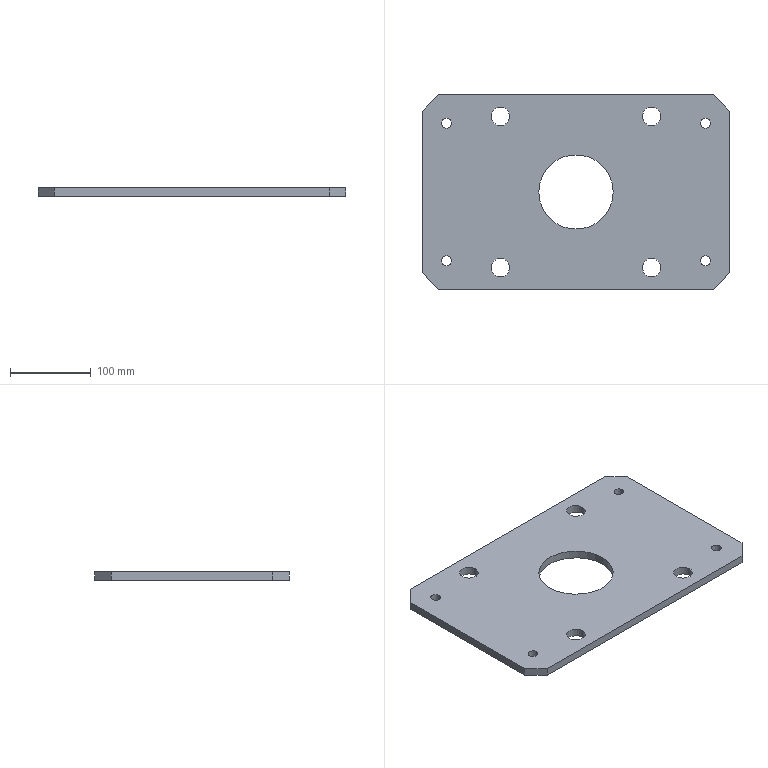Part | SolidWorks | features BaseBody 1 | 1 solid | 28 faces | box 380 x 240 x 10 mm | volume 816381 mm3 | cylinder 18 | plane 10 | commonest cylinder face diameters 12 x8 23 x8 92 x2
STEP:
#1=CARTESIAN_POINT('',(-154.,85.,10.));
#2=VERTEX_POINT('',#1);
#3=CARTESIAN_POINT('',(-166.,85.,10.));
#4=VERTEX_POINT('',#3);
#5=CARTESIAN_POINT('',(-160.,85.,10.));
#6=DIRECTION('',(0.,0.,-1.));
#7=DIRECTION('',(-1.,0.,0.));
#8=AXIS2_PLACEMENT_3D('',#5,#6,#7);
#9=CIRCLE('',#8,6.);
#10=EDGE_CURVE('',#2,#4,#9,.T.);
#11=ORIENTED_EDGE('',*,*,#10,.F.);
#12=CARTESIAN_POINT('',(-154.,85.,0.));
#13=VERTEX_POINT('',#12);
#14=CARTESIAN_POINT('',(-154.,85.,10.));
#15=DIRECTION('',(0.,0.,-1.));
#16=VECTOR('',#15,1000.);
#17=LINE('',#14,#16);
#18=EDGE_CURVE('',#2,#13,#17,.T.);
#19=ORIENTED_EDGE('',*,*,#18,.T.);
#20=CARTESIAN_POINT('',(-166.,85.,0.));
#21=VERTEX_POINT('',#20);
#22=CARTESIAN_POINT('',(-160.,85.,0.));
#23=DIRECTION('',(0.,0.,-1.));
#24=DIRECTION('',(-1.,0.,0.));
#25=AXIS2_PLACEMENT_3D('',#22,#23,#24);
#26=CIRCLE('',#25,6.);
#27=EDGE_CURVE('',#13,#21,#26,.T.);
#28=ORIENTED_EDGE('',*,*,#27,.T.);
#29=CARTESIAN_POINT('',(-166.,85.,10.));
#30=DIRECTION('',(0.,0.,-1.));
#31=VECTOR('',#30,1000.);
#32=LINE('',#29,#31);
#33=EDGE_CURVE('',#4,#21,#32,.T.);
#34=ORIENTED_EDGE('',*,*,#33,.F.);
#35=EDGE_LOOP('',(#11,#19,#28,#34));
#36=FACE_OUTER_BOUND('',#35,.T.);
#37=CARTESIAN_POINT('',(-160.,85.,10.));
#38=DIRECTION('',(0.,0.,-1.));
#39=DIRECTION('',(-1.,0.,0.));
#40=AXIS2_PLACEMENT_3D('',#37,#38,#39);
#41=CYLINDRICAL_SURFACE('',#40,6.);
#42=ADVANCED_FACE('',(#36),#41,.F.);
#43=CARTESIAN_POINT('',(-154.,-85.,10.));
#44=VERTEX_POINT('',#43);
#45=CARTESIAN_POINT('',(-166.,-85.,10.));
#46=VERTEX_POINT('',#45);
#47=CARTESIAN_POINT('',(-160.,-85.,10.));
#48=DIRECTION('',(0.,0.,-1.));
#49=DIRECTION('',(-1.,0.,0.));
#50=AXIS2_PLACEMENT_3D('',#47,#48,#49);
#51=CIRCLE('',#50,6.);
#52=EDGE_CURVE('',#44,#46,#51,.T.);
#53=ORIENTED_EDGE('',*,*,#52,.F.);
#54=CARTESIAN_POINT('',(-154.,-85.,0.));
#55=VERTEX_POINT('',#54);
#56=CARTESIAN_POINT('',(-154.,-85.,10.));
#57=DIRECTION('',(0.,0.,-1.));
#58=VECTOR('',#57,1000.);
#59=LINE('',#56,#58);
#60=EDGE_CURVE('',#44,#55,#59,.T.);
#61=ORIENTED_EDGE('',*,*,#60,.T.);
#62=CARTESIAN_POINT('',(-166.,-85.,0.));
#63=VERTEX_POINT('',#62);
#64=CARTESIAN_POINT('',(-160.,-85.,0.));
#65=DIRECTION('',(0.,0.,-1.));
#66=DIRECTION('',(-1.,0.,0.));
#67=AXIS2_PLACEMENT_3D('',#64,#65,#66);
#68=CIRCLE('',#67,6.);
#69=EDGE_CURVE('',#55,#63,#68,.T.);
#70=ORIENTED_EDGE('',*,*,#69,.T.);
#71=CARTESIAN_POINT('',(-166.,-85.,10.));
#72=DIRECTION('',(0.,0.,-1.));
#73=VECTOR('',#72,1000.);
#74=LINE('',#71,#73);
#75=EDGE_CURVE('',#46,#63,#74,.T.);
#76=ORIENTED_EDGE('',*,*,#75,.F.);
#77=EDGE_LOOP('',(#53,#61,#70,#76));
#78=FACE_OUTER_BOUND('',#77,.T.);
#79=CARTESIAN_POINT('',(-160.,-85.,10.));
#80=DIRECTION('',(0.,0.,-1.));
#81=DIRECTION('',(-1.,0.,0.));
#82=AXIS2_PLACEMENT_3D('',#79,#80,#81);
#83=CYLINDRICAL_SURFACE('',#82,6.);
#84=ADVANCED_FACE('',(#78),#83,.F.);
#85=CARTESIAN_POINT('',(166.,85.,10.));
#86=VERTEX_POINT('',#85);
#87=CARTESIAN_POINT('',(154.,85.,10.));
#88=VERTEX_POINT('',#87);
#89=CARTESIAN_POINT('',(160.,85.,10.));
#90=DIRECTION('',(0.,0.,-1.));
#91=DIRECTION('',(-1.,0.,0.));
#92=AXIS2_PLACEMENT_3D('',#89,#90,#91);
#93=CIRCLE('',#92,6.);
#94=EDGE_CURVE('',#86,#88,#93,.T.);
#95=ORIENTED_EDGE('',*,*,#94,.F.);
#96=CARTESIAN_POINT('',(166.,85.,0.));
#97=VERTEX_POINT('',#96);
#98=CARTESIAN_POINT('',(166.,85.,10.));
#99=DIRECTION('',(0.,0.,-1.));
#100=VECTOR('',#99,1000.);
#101=LINE('',#98,#100);
#102=EDGE_CURVE('',#86,#97,#101,.T.);
#103=ORIENTED_EDGE('',*,*,#102,.T.);
#104=CARTESIAN_POINT('',(154.,85.,0.));
#105=VERTEX_POINT('',#104);
#106=CARTESIAN_POINT('',(160.,85.,0.));
#107=DIRECTION('',(0.,0.,-1.));
#108=DIRECTION('',(-1.,0.,0.));
#109=AXIS2_PLACEMENT_3D('',#106,#107,#108);
#110=CIRCLE('',#109,6.);
#111=EDGE_CURVE('',#97,#105,#110,.T.);
#112=ORIENTED_EDGE('',*,*,#111,.T.);
#113=CARTESIAN_POINT('',(154.,85.,10.));
#114=DIRECTION('',(0.,0.,-1.));
#115=VECTOR('',#114,1000.);
#116=LINE('',#113,#115);
#117=EDGE_CURVE('',#88,#105,#116,.T.);
#118=ORIENTED_EDGE('',*,*,#117,.F.);
#119=EDGE_LOOP('',(#95,#103,#112,#118));
#120=FACE_OUTER_BOUND('',#119,.T.);
#121=CARTESIAN_POINT('',(160.,85.,10.));
#122=DIRECTION('',(0.,0.,-1.));
#123=DIRECTION('',(-1.,0.,0.));
#124=AXIS2_PLACEMENT_3D('',#121,#122,#123);
#125=CYLINDRICAL_SURFACE('',#124,6.);
#126=ADVANCED_FACE('',(#120),#125,.F.);
#127=CARTESIAN_POINT('',(166.,-85.,10.));
#128=VERTEX_POINT('',#127);
#129=CARTESIAN_POINT('',(154.,-85.,10.));
#130=VERTEX_POINT('',#129);
#131=CARTESIAN_POINT('',(160.,-85.,10.));
#132=DIRECTION('',(0.,0.,-1.));
#133=DIRECTION('',(-1.,0.,0.));
#134=AXIS2_PLACEMENT_3D('',#131,#132,#133);
#135=CIRCLE('',#134,6.);
#136=EDGE_CURVE('',#128,#130,#135,.T.);
#137=ORIENTED_EDGE('',*,*,#136,.F.);
#138=CARTESIAN_POINT('',(166.,-85.,0.));
#139=VERTEX_POINT('',#138);
#140=CARTESIAN_POINT('',(166.,-85.,10.));
#141=DIRECTION('',(0.,0.,-1.));
#142=VECTOR('',#141,1000.);
#143=LINE('',#140,#142);
#144=EDGE_CURVE('',#128,#139,#143,.T.);
#145=ORIENTED_EDGE('',*,*,#144,.T.);
#146=CARTESIAN_POINT('',(154.,-85.,0.));
#147=VERTEX_POINT('',#146);
#148=CARTESIAN_POINT('',(160.,-85.,0.));
#149=DIRECTION('',(0.,0.,-1.));
#150=DIRECTION('',(-1.,0.,0.));
#151=AXIS2_PLACEMENT_3D('',#148,#149,#150);
#152=CIRCLE('',#151,6.);
#153=EDGE_CURVE('',#139,#147,#152,.T.);
#154=ORIENTED_EDGE('',*,*,#153,.T.);
#155=CARTESIAN_POINT('',(154.,-85.,10.));
#156=DIRECTION('',(0.,0.,-1.));
#157=VECTOR('',#156,1000.);
#158=LINE('',#155,#157);
#159=EDGE_CURVE('',#130,#147,#158,.T.);
#160=ORIENTED_EDGE('',*,*,#159,.F.);
#161=EDGE_LOOP('',(#137,#145,#154,#160));
#162=FACE_OUTER_BOUND('',#161,.T.);
#163=CARTESIAN_POINT('',(160.,-85.,10.));
#164=DIRECTION('',(0.,0.,-1.));
#165=DIRECTION('',(-1.,0.,0.));
#166=AXIS2_PLACEMENT_3D('',#163,#164,#165);
#167=CYLINDRICAL_SURFACE('',#166,6.);
#168=ADVANCED_FACE('',(#162),#167,.F.);
#169=CARTESIAN_POINT('',(-82.,93.5,10.));
#170=VERTEX_POINT('',#169);
#171=CARTESIAN_POINT('',(-105.,93.5,10.));
#172=VERTEX_POINT('',#171);
#173=CARTESIAN_POINT('',(-93.5,93.5,10.));
#174=DIRECTION('',(0.,0.,-1.));
#175=DIRECTION('',(-1.,0.,0.));
#176=AXIS2_PLACEMENT_3D('',#173,#174,#175);
#177=CIRCLE('',#176,11.5);
#178=EDGE_CURVE('',#170,#172,#177,.T.);
#179=ORIENTED_EDGE('',*,*,#178,.F.);
#180=CARTESIAN_POINT('',(-82.,93.5,0.));
#181=VERTEX_POINT('',#180);
#182=CARTESIAN_POINT('',(-82.,93.5,10.));
#183=DIRECTION('',(0.,0.,-1.));
#184=VECTOR('',#183,1000.);
#185=LINE('',#182,#184);
#186=EDGE_CURVE('',#170,#181,#185,.T.);
#187=ORIENTED_EDGE('',*,*,#186,.T.);
#188=CARTESIAN_POINT('',(-105.,93.5,0.));
#189=VERTEX_POINT('',#188);
#190=CARTESIAN_POINT('',(-93.5,93.5,0.));
#191=DIRECTION('',(0.,0.,-1.));
#192=DIRECTION('',(-1.,0.,0.));
#193=AXIS2_PLACEMENT_3D('',#190,#191,#192);
#194=CIRCLE('',#193,11.5);
#195=EDGE_CURVE('',#181,#189,#194,.T.);
#196=ORIENTED_EDGE('',*,*,#195,.T.);
#197=CARTESIAN_POINT('',(-105.,93.5,10.));
#198=DIRECTION('',(0.,0.,-1.));
#199=VECTOR('',#198,1000.);
#200=LINE('',#197,#199);
#201=EDGE_CURVE('',#172,#189,#200,.T.);
#202=ORIENTED_EDGE('',*,*,#201,.F.);
#203=EDGE_LOOP('',(#179,#187,#196,#202));
#204=FACE_OUTER_BOUND('',#203,.T.);
#205=CARTESIAN_POINT('',(-93.5,93.5,10.));
#206=DIRECTION('',(0.,0.,-1.));
#207=DIRECTION('',(-1.,0.,0.));
#208=AXIS2_PLACEMENT_3D('',#205,#206,#207);
#209=CYLINDRICAL_SURFACE('',#208,11.5);
#210=ADVANCED_FACE('',(#204),#209,.F.);
#211=CARTESIAN_POINT('',(-82.,-93.5,10.));
#212=VERTEX_POINT('',#211);
#213=CARTESIAN_POINT('',(-105.,-93.5,10.));
#214=VERTEX_POINT('',#213);
#215=CARTESIAN_POINT('',(-93.5,-93.5,10.));
#216=DIRECTION('',(0.,0.,-1.));
#217=DIRECTION('',(-1.,0.,0.));
#218=AXIS2_PLACEMENT_3D('',#215,#216,#217);
#219=CIRCLE('',#218,11.5);
#220=EDGE_CURVE('',#212,#214,#219,.T.);
#221=ORIENTED_EDGE('',*,*,#220,.F.);
#222=CARTESIAN_POINT('',(-82.,-93.5,0.));
#223=VERTEX_POINT('',#222);
#224=CARTESIAN_POINT('',(-82.,-93.5,10.));
#225=DIRECTION('',(0.,0.,-1.));
#226=VECTOR('',#225,1000.);
#227=LINE('',#224,#226);
#228=EDGE_CURVE('',#212,#223,#227,.T.);
#229=ORIENTED_EDGE('',*,*,#228,.T.);
#230=CARTESIAN_POINT('',(-105.,-93.5,0.));
#231=VERTEX_POINT('',#230);
#232=CARTESIAN_POINT('',(-93.5,-93.5,0.));
#233=DIRECTION('',(0.,0.,-1.));
#234=DIRECTION('',(-1.,0.,0.));
#235=AXIS2_PLACEMENT_3D('',#232,#233,#234);
#236=CIRCLE('',#235,11.5);
#237=EDGE_CURVE('',#223,#231,#236,.T.);
#238=ORIENTED_EDGE('',*,*,#237,.T.);
#239=CARTESIAN_POINT('',(-105.,-93.5,10.));
#240=DIRECTION('',(0.,0.,-1.));
#241=VECTOR('',#240,1000.);
#242=LINE('',#239,#241);
#243=EDGE_CURVE('',#214,#231,#242,.T.);
#244=ORIENTED_EDGE('',*,*,#243,.F.);
#245=EDGE_LOOP('',(#221,#229,#238,#244));
#246=FACE_OUTER_BOUND('',#245,.T.);
#247=CARTESIAN_POINT('',(-93.5,-93.5,10.));
#248=DIRECTION('',(0.,0.,-1.));
#249=DIRECTION('',(-1.,0.,0.));
#250=AXIS2_PLACEMENT_3D('',#247,#248,#249);
#251=CYLINDRICAL_SURFACE('',#250,11.5);
#252=ADVANCED_FACE('',(#246),#251,.F.);
#253=CARTESIAN_POINT('',(105.,93.5,10.));
#254=VERTEX_POINT('',#253);
#255=CARTESIAN_POINT('',(82.,93.5,10.));
#256=VERTEX_POINT('',#255);
#257=CARTESIAN_POINT('',(93.5,93.5,10.));
#258=DIRECTION('',(0.,0.,-1.));
#259=DIRECTION('',(-1.,0.,0.));
#260=AXIS2_PLACEMENT_3D('',#257,#258,#259);
#261=CIRCLE('',#260,11.5);
#262=EDGE_CURVE('',#254,#256,#261,.T.);
#263=ORIENTED_EDGE('',*,*,#262,.F.);
#264=CARTESIAN_POINT('',(105.,93.5,0.));
#265=VERTEX_POINT('',#264);
#266=CARTESIAN_POINT('',(105.,93.5,10.));
#267=DIRECTION('',(0.,0.,-1.));
#268=VECTOR('',#267,1000.);
#269=LINE('',#266,#268);
#270=EDGE_CURVE('',#254,#265,#269,.T.);
#271=ORIENTED_EDGE('',*,*,#270,.T.);
#272=CARTESIAN_POINT('',(82.,93.5,0.));
#273=VERTEX_POINT('',#272);
#274=CARTESIAN_POINT('',(93.5,93.5,0.));
#275=DIRECTION('',(0.,0.,-1.));
#276=DIRECTION('',(-1.,0.,0.));
#277=AXIS2_PLACEMENT_3D('',#274,#275,#276);
#278=CIRCLE('',#277,11.5);
#279=EDGE_CURVE('',#265,#273,#278,.T.);
#280=ORIENTED_EDGE('',*,*,#279,.T.);
#281=CARTESIAN_POINT('',(82.,93.5,10.));
#282=DIRECTION('',(0.,0.,-1.));
#283=VECTOR('',#282,1000.);
#284=LINE('',#281,#283);
#285=EDGE_CURVE('',#256,#273,#284,.T.);
#286=ORIENTED_EDGE('',*,*,#285,.F.);
#287=EDGE_LOOP('',(#263,#271,#280,#286));
#288=FACE_OUTER_BOUND('',#287,.T.);
#289=CARTESIAN_POINT('',(93.5,93.5,10.));
#290=DIRECTION('',(0.,0.,-1.));
#291=DIRECTION('',(-1.,0.,0.));
#292=AXIS2_PLACEMENT_3D('',#289,#290,#291);
#293=CYLINDRICAL_SURFACE('',#292,11.5);
#294=ADVANCED_FACE('',(#288),#293,.F.);
#295=CARTESIAN_POINT('',(105.,-93.5,10.));
#296=VERTEX_POINT('',#295);
#297=CARTESIAN_POINT('',(82.,-93.5,10.));
#298=VERTEX_POINT('',#297);
#299=CARTESIAN_POINT('',(93.5,-93.5,10.));
#300=DIRECTION('',(0.,0.,-1.));
#301=DIRECTION('',(-1.,0.,0.));
#302=AXIS2_PLACEMENT_3D('',#299,#300,#301);
#303=CIRCLE('',#302,11.5);
#304=EDGE_CURVE('',#296,#298,#303,.T.);
#305=ORIENTED_EDGE('',*,*,#304,.F.);
#306=CARTESIAN_POINT('',(105.,-93.5,0.));
#307=VERTEX_POINT('',#306);
#308=CARTESIAN_POINT('',(105.,-93.5,10.));
#309=DIRECTION('',(0.,0.,-1.));
#310=VECTOR('',#309,1000.);
#311=LINE('',#308,#310);
#312=EDGE_CURVE('',#296,#307,#311,.T.);
#313=ORIENTED_EDGE('',*,*,#312,.T.);
#314=CARTESIAN_POINT('',(82.,-93.5,0.));
#315=VERTEX_POINT('',#314);
#316=CARTESIAN_POINT('',(93.5,-93.5,0.));
#317=DIRECTION('',(0.,0.,-1.));
#318=DIRECTION('',(-1.,0.,0.));
#319=AXIS2_PLACEMENT_3D('',#316,#317,#318);
#320=CIRCLE('',#319,11.5);
#321=EDGE_CURVE('',#307,#315,#320,.T.);
#322=ORIENTED_EDGE('',*,*,#321,.T.);
#323=CARTESIAN_POINT('',(82.,-93.5,10.));
#324=DIRECTION('',(0.,0.,-1.));
#325=VECTOR('',#324,1000.);
#326=LINE('',#323,#325);
#327=EDGE_CURVE('',#298,#315,#326,.T.);
#328=ORIENTED_EDGE('',*,*,#327,.F.);
#329=EDGE_LOOP('',(#305,#313,#322,#328));
#330=FACE_OUTER_BOUND('',#329,.T.);
#331=CARTESIAN_POINT('',(93.5,-93.5,10.));
#332=DIRECTION('',(0.,0.,-1.));
#333=DIRECTION('',(-1.,0.,0.));
#334=AXIS2_PLACEMENT_3D('',#331,#332,#333);
#335=CYLINDRICAL_SURFACE('',#334,11.5);
#336=ADVANCED_FACE('',(#330),#335,.F.);
#337=CARTESIAN_POINT('',(46.,0.,10.));
#338=VERTEX_POINT('',#337);
#339=CARTESIAN_POINT('',(-46.,0.,10.));
#340=VERTEX_POINT('',#339);
#341=CARTESIAN_POINT('',(0.,0.,10.));
#342=DIRECTION('',(0.,0.,-1.));
#343=DIRECTION('',(-1.,0.,0.));
#344=AXIS2_PLACEMENT_3D('',#341,#342,#343);
#345=CIRCLE('',#344,46.);
#346=EDGE_CURVE('',#338,#340,#345,.T.);
#347=ORIENTED_EDGE('',*,*,#346,.F.);
#348=CARTESIAN_POINT('',(46.,0.,0.));
#349=VERTEX_POINT('',#348);
#350=CARTESIAN_POINT('',(46.,0.,10.));
#351=DIRECTION('',(0.,0.,-1.));
#352=VECTOR('',#351,1000.);
#353=LINE('',#350,#352);
#354=EDGE_CURVE('',#338,#349,#353,.T.);
#355=ORIENTED_EDGE('',*,*,#354,.T.);
#356=CARTESIAN_POINT('',(-46.,0.,0.));
#357=VERTEX_POINT('',#356);
#358=CARTESIAN_POINT('',(0.,0.,0.));
#359=DIRECTION('',(0.,0.,-1.));
#360=DIRECTION('',(-1.,0.,0.));
#361=AXIS2_PLACEMENT_3D('',#358,#359,#360);
#362=CIRCLE('',#361,46.);
#363=EDGE_CURVE('',#349,#357,#362,.T.);
#364=ORIENTED_EDGE('',*,*,#363,.T.);
#365=CARTESIAN_POINT('',(-46.,0.,10.));
#366=DIRECTION('',(0.,0.,-1.));
#367=VECTOR('',#366,1000.);
#368=LINE('',#365,#367);
#369=EDGE_CURVE('',#340,#357,#368,.T.);
#370=ORIENTED_EDGE('',*,*,#369,.F.);
#371=EDGE_LOOP('',(#347,#355,#364,#370));
#372=FACE_OUTER_BOUND('',#371,.T.);
#373=CARTESIAN_POINT('',(0.,0.,10.));
#374=DIRECTION('',(0.,0.,-1.));
#375=DIRECTION('',(-1.,0.,0.));
#376=AXIS2_PLACEMENT_3D('',#373,#374,#375);
#377=CYLINDRICAL_SURFACE('',#376,46.);
#378=ADVANCED_FACE('',(#372),#377,.F.);
#379=CARTESIAN_POINT('',(-160.,85.,0.));
#380=DIRECTION('',(0.,0.,-1.));
#381=DIRECTION('',(-1.,0.,0.));
#382=AXIS2_PLACEMENT_3D('',#379,#380,#381);
#383=CIRCLE('',#382,6.);
#384=EDGE_CURVE('',#21,#13,#383,.T.);
#385=ORIENTED_EDGE('',*,*,#384,.F.);
#386=ORIENTED_EDGE('',*,*,#27,.F.);
#387=EDGE_LOOP('',(#385,#386));
#388=FACE_BOUND('',#387,.T.);
#389=CARTESIAN_POINT('',(-160.,-85.,0.));
#390=DIRECTION('',(0.,0.,-1.));
#391=DIRECTION('',(-1.,0.,0.));
#392=AXIS2_PLACEMENT_3D('',#389,#390,#391);
#393=CIRCLE('',#392,6.);
#394=EDGE_CURVE('',#63,#55,#393,.T.);
#395=ORIENTED_EDGE('',*,*,#394,.F.);
#396=ORIENTED_EDGE('',*,*,#69,.F.);
#397=EDGE_LOOP('',(#395,#396));
#398=FACE_BOUND('',#397,.T.);
#399=CARTESIAN_POINT('',(160.,85.,0.));
#400=DIRECTION('',(0.,0.,-1.));
#401=DIRECTION('',(-1.,0.,0.));
#402=AXIS2_PLACEMENT_3D('',#399,#400,#401);
#403=CIRCLE('',#402,6.);
#404=EDGE_CURVE('',#105,#97,#403,.T.);
#405=ORIENTED_EDGE('',*,*,#404,.F.);
#406=ORIENTED_EDGE('',*,*,#111,.F.);
#407=EDGE_LOOP('',(#405,#406));
#408=FACE_BOUND('',#407,.T.);
#409=CARTESIAN_POINT('',(160.,-85.,0.));
#410=DIRECTION('',(0.,0.,-1.));
#411=DIRECTION('',(-1.,0.,0.));
#412=AXIS2_PLACEMENT_3D('',#409,#410,#411);
#413=CIRCLE('',#412,6.);
#414=EDGE_CURVE('',#147,#139,#413,.T.);
#415=ORIENTED_EDGE('',*,*,#414,.F.);
#416=ORIENTED_EDGE('',*,*,#153,.F.);
#417=EDGE_LOOP('',(#415,#416));
#418=FACE_BOUND('',#417,.T.);
#419=CARTESIAN_POINT('',(-93.5,93.5,0.));
#420=DIRECTION('',(0.,0.,-1.));
#421=DIRECTION('',(-1.,0.,0.));
#422=AXIS2_PLACEMENT_3D('',#419,#420,#421);
#423=CIRCLE('',#422,11.5);
#424=EDGE_CURVE('',#189,#181,#423,.T.);
#425=ORIENTED_EDGE('',*,*,#424,.F.);
#426=ORIENTED_EDGE('',*,*,#195,.F.);
#427=EDGE_LOOP('',(#425,#426));
#428=FACE_BOUND('',#427,.T.);
#429=CARTESIAN_POINT('',(-93.5,-93.5,0.));
#430=DIRECTION('',(0.,0.,-1.));
#431=DIRECTION('',(-1.,0.,0.));
#432=AXIS2_PLACEMENT_3D('',#429,#430,#431);
#433=CIRCLE('',#432,11.5);
#434=EDGE_CURVE('',#231,#223,#433,.T.);
#435=ORIENTED_EDGE('',*,*,#434,.F.);
#436=ORIENTED_EDGE('',*,*,#237,.F.);
#437=EDGE_LOOP('',(#435,#436));
#438=FACE_BOUND('',#437,.T.);
#439=CARTESIAN_POINT('',(93.5,93.5,0.));
#440=DIRECTION('',(0.,0.,-1.));
#441=DIRECTION('',(-1.,0.,0.));
#442=AXIS2_PLACEMENT_3D('',#439,#440,#441);
#443=CIRCLE('',#442,11.5);
#444=EDGE_CURVE('',#273,#265,#443,.T.);
#445=ORIENTED_EDGE('',*,*,#444,.F.);
#446=ORIENTED_EDGE('',*,*,#279,.F.);
#447=EDGE_LOOP('',(#445,#446));
#448=FACE_BOUND('',#447,.T.);
#449=CARTESIAN_POINT('',(93.5,-93.5,0.));
#450=DIRECTION('',(0.,0.,-1.));
#451=DIRECTION('',(-1.,0.,0.));
#452=AXIS2_PLACEMENT_3D('',#449,#450,#451);
#453=CIRCLE('',#452,11.5);
#454=EDGE_CURVE('',#315,#307,#453,.T.);
#455=ORIENTED_EDGE('',*,*,#454,.F.);
#456=ORIENTED_EDGE('',*,*,#321,.F.);
#457=EDGE_LOOP('',(#455,#456));
#458=FACE_BOUND('',#457,.T.);
#459=CARTESIAN_POINT('',(0.,0.,0.));
#460=DIRECTION('',(0.,0.,-1.));
#461=DIRECTION('',(-1.,0.,0.));
#462=AXIS2_PLACEMENT_3D('',#459,#460,#461);
#463=CIRCLE('',#462,46.);
#464=EDGE_CURVE('',#357,#349,#463,.T.);
#465=ORIENTED_EDGE('',*,*,#464,.F.);
#466=ORIENTED_EDGE('',*,*,#363,.F.);
#467=EDGE_LOOP('',(#465,#466));
#468=FACE_BOUND('',#467,.T.);
#469=CARTESIAN_POINT('',(170.,-120.,0.));
#470=VERTEX_POINT('',#469);
#471=CARTESIAN_POINT('',(190.,-100.,0.));
#472=VERTEX_POINT('',#471);
#473=CARTESIAN_POINT('',(170.,-120.,0.));
#474=DIRECTION('',(0.7071,0.7071,0.));
#475=VECTOR('',#474,1000.);
#476=LINE('',#473,#475);
#477=EDGE_CURVE('',#470,#472,#476,.T.);
#478=ORIENTED_EDGE('',*,*,#477,.F.);
#479=CARTESIAN_POINT('',(-170.,-120.,0.));
#480=VERTEX_POINT('',#479);
#481=CARTESIAN_POINT('',(0.,-120.,0.));
#482=DIRECTION('',(1.,0.,0.));
#483=VECTOR('',#482,1000.);
#484=LINE('',#481,#483);
#485=EDGE_CURVE('',#480,#470,#484,.T.);
#486=ORIENTED_EDGE('',*,*,#485,.F.);
#487=CARTESIAN_POINT('',(-190.,-100.,0.));
#488=VERTEX_POINT('',#487);
#489=CARTESIAN_POINT('',(-190.,-100.,0.));
#490=DIRECTION('',(0.7071,-0.7071,0.));
#491=VECTOR('',#490,1000.);
#492=LINE('',#489,#491);
#493=EDGE_CURVE('',#488,#480,#492,.T.);
#494=ORIENTED_EDGE('',*,*,#493,.F.);
#495=CARTESIAN_POINT('',(-190.,100.,0.));
#496=VERTEX_POINT('',#495);
#497=CARTESIAN_POINT('',(-190.,0.,0.));
#498=DIRECTION('',(0.,-1.,0.));
#499=VECTOR('',#498,1000.);
#500=LINE('',#497,#499);
#501=EDGE_CURVE('',#496,#488,#500,.T.);
#502=ORIENTED_EDGE('',*,*,#501,.F.);
#503=CARTESIAN_POINT('',(-170.,120.,0.));
#504=VERTEX_POINT('',#503);
#505=CARTESIAN_POINT('',(-170.,120.,0.));
#506=DIRECTION('',(-0.7071,-0.7071,0.));
#507=VECTOR('',#506,1000.);
#508=LINE('',#505,#507);
#509=EDGE_CURVE('',#504,#496,#508,.T.);
#510=ORIENTED_EDGE('',*,*,#509,.F.);
#511=CARTESIAN_POINT('',(170.,120.,0.));
#512=VERTEX_POINT('',#511);
#513=CARTESIAN_POINT('',(0.,120.,0.));
#514=DIRECTION('',(-1.,0.,0.));
#515=VECTOR('',#514,1000.);
#516=LINE('',#513,#515);
#517=EDGE_CURVE('',#512,#504,#516,.T.);
#518=ORIENTED_EDGE('',*,*,#517,.F.);
#519=CARTESIAN_POINT('',(190.,100.,0.));
#520=VERTEX_POINT('',#519);
#521=CARTESIAN_POINT('',(190.,100.,0.));
#522=DIRECTION('',(-0.7071,0.7071,0.));
#523=VECTOR('',#522,1000.);
#524=LINE('',#521,#523);
#525=EDGE_CURVE('',#520,#512,#524,.T.);
#526=ORIENTED_EDGE('',*,*,#525,.F.);
#527=CARTESIAN_POINT('',(190.,0.,0.));
#528=DIRECTION('',(0.,1.,0.));
#529=VECTOR('',#528,1000.);
#530=LINE('',#527,#529);
#531=EDGE_CURVE('',#472,#520,#530,.T.);
#532=ORIENTED_EDGE('',*,*,#531,.F.);
#533=EDGE_LOOP('',(#478,#486,#494,#502,#510,#518,#526,#532));
#534=FACE_OUTER_BOUND('',#533,.T.);
#535=CARTESIAN_POINT('',(0.,0.,0.));
#536=DIRECTION('',(0.,0.,1.));
#537=DIRECTION('',(1.,0.,0.));
#538=AXIS2_PLACEMENT_3D('',#535,#536,#537);
#539=PLANE('',#538);
#540=ADVANCED_FACE('',(#388,#398,#408,#418,#428,#438,#448,#458,#468,#534),#539,.F.);
#541=ORIENTED_EDGE('',*,*,#18,.F.);
#542=CARTESIAN_POINT('',(-160.,85.,10.));
#543=DIRECTION('',(0.,0.,-1.));
#544=DIRECTION('',(-1.,0.,0.));
#545=AXIS2_PLACEMENT_3D('',#542,#543,#544);
#546=CIRCLE('',#545,6.);
#547=EDGE_CURVE('',#4,#2,#546,.T.);
#548=ORIENTED_EDGE('',*,*,#547,.F.);
#549=ORIENTED_EDGE('',*,*,#33,.T.);
#550=ORIENTED_EDGE('',*,*,#384,.T.);
#551=EDGE_LOOP('',(#541,#548,#549,#550));
#552=FACE_OUTER_BOUND('',#551,.T.);
#553=CARTESIAN_POINT('',(-160.,85.,10.));
#554=DIRECTION('',(0.,0.,-1.));
#555=DIRECTION('',(-1.,0.,0.));
#556=AXIS2_PLACEMENT_3D('',#553,#554,#555);
#557=CYLINDRICAL_SURFACE('',#556,6.);
#558=ADVANCED_FACE('',(#552),#557,.F.);
#559=ORIENTED_EDGE('',*,*,#60,.F.);
#560=CARTESIAN_POINT('',(-160.,-85.,10.));
#561=DIRECTION('',(0.,0.,-1.));
#562=DIRECTION('',(-1.,0.,0.));
#563=AXIS2_PLACEMENT_3D('',#560,#561,#562);
#564=CIRCLE('',#563,6.);
#565=EDGE_CURVE('',#46,#44,#564,.T.);
#566=ORIENTED_EDGE('',*,*,#565,.F.);
#567=ORIENTED_EDGE('',*,*,#75,.T.);
#568=ORIENTED_EDGE('',*,*,#394,.T.);
#569=EDGE_LOOP('',(#559,#566,#567,#568));
#570=FACE_OUTER_BOUND('',#569,.T.);
#571=CARTESIAN_POINT('',(-160.,-85.,10.));
#572=DIRECTION('',(0.,0.,-1.));
#573=DIRECTION('',(-1.,0.,0.));
#574=AXIS2_PLACEMENT_3D('',#571,#572,#573);
#575=CYLINDRICAL_SURFACE('',#574,6.);
#576=ADVANCED_FACE('',(#570),#575,.F.);
#577=ORIENTED_EDGE('',*,*,#102,.F.);
#578=CARTESIAN_POINT('',(160.,85.,10.));
#579=DIRECTION('',(0.,0.,-1.));
#580=DIRECTION('',(-1.,0.,0.));
#581=AXIS2_PLACEMENT_3D('',#578,#579,#580);
#582=CIRCLE('',#581,6.);
#583=EDGE_CURVE('',#88,#86,#582,.T.);
#584=ORIENTED_EDGE('',*,*,#583,.F.);
#585=ORIENTED_EDGE('',*,*,#117,.T.);
#586=ORIENTED_EDGE('',*,*,#404,.T.);
#587=EDGE_LOOP('',(#577,#584,#585,#586));
#588=FACE_OUTER_BOUND('',#587,.T.);
#589=CARTESIAN_POINT('',(160.,85.,10.));
#590=DIRECTION('',(0.,0.,-1.));
#591=DIRECTION('',(-1.,0.,0.));
#592=AXIS2_PLACEMENT_3D('',#589,#590,#591);
#593=CYLINDRICAL_SURFACE('',#592,6.);
#594=ADVANCED_FACE('',(#588),#593,.F.);
#595=ORIENTED_EDGE('',*,*,#144,.F.);
#596=CARTESIAN_POINT('',(160.,-85.,10.));
#597=DIRECTION('',(0.,0.,-1.));
#598=DIRECTION('',(-1.,0.,0.));
#599=AXIS2_PLACEMENT_3D('',#596,#597,#598);
#600=CIRCLE('',#599,6.);
#601=EDGE_CURVE('',#130,#128,#600,.T.);
#602=ORIENTED_EDGE('',*,*,#601,.F.);
#603=ORIENTED_EDGE('',*,*,#159,.T.);
#604=ORIENTED_EDGE('',*,*,#414,.T.);
#605=EDGE_LOOP('',(#595,#602,#603,#604));
#606=FACE_OUTER_BOUND('',#605,.T.);
#607=CARTESIAN_POINT('',(160.,-85.,10.));
#608=DIRECTION('',(0.,0.,-1.));
#609=DIRECTION('',(-1.,0.,0.));
#610=AXIS2_PLACEMENT_3D('',#607,#608,#609);
#611=CYLINDRICAL_SURFACE('',#610,6.);
#612=ADVANCED_FACE('',(#606),#611,.F.);
#613=ORIENTED_EDGE('',*,*,#186,.F.);
#614=CARTESIAN_POINT('',(-93.5,93.5,10.));
#615=DIRECTION('',(0.,0.,-1.));
#616=DIRECTION('',(-1.,0.,0.));
#617=AXIS2_PLACEMENT_3D('',#614,#615,#616);
#618=CIRCLE('',#617,11.5);
#619=EDGE_CURVE('',#172,#170,#618,.T.);
#620=ORIENTED_EDGE('',*,*,#619,.F.);
#621=ORIENTED_EDGE('',*,*,#201,.T.);
#622=ORIENTED_EDGE('',*,*,#424,.T.);
#623=EDGE_LOOP('',(#613,#620,#621,#622));
#624=FACE_OUTER_BOUND('',#623,.T.);
#625=CARTESIAN_POINT('',(-93.5,93.5,10.));
#626=DIRECTION('',(0.,0.,-1.));
#627=DIRECTION('',(-1.,0.,0.));
#628=AXIS2_PLACEMENT_3D('',#625,#626,#627);
#629=CYLINDRICAL_SURFACE('',#628,11.5);
#630=ADVANCED_FACE('',(#624),#629,.F.);
#631=ORIENTED_EDGE('',*,*,#228,.F.);
#632=CARTESIAN_POINT('',(-93.5,-93.5,10.));
#633=DIRECTION('',(0.,0.,-1.));
#634=DIRECTION('',(-1.,0.,0.));
#635=AXIS2_PLACEMENT_3D('',#632,#633,#634);
#636=CIRCLE('',#635,11.5);
#637=EDGE_CURVE('',#214,#212,#636,.T.);
#638=ORIENTED_EDGE('',*,*,#637,.F.);
#639=ORIENTED_EDGE('',*,*,#243,.T.);
#640=ORIENTED_EDGE('',*,*,#434,.T.);
#641=EDGE_LOOP('',(#631,#638,#639,#640));
#642=FACE_OUTER_BOUND('',#641,.T.);
#643=CARTESIAN_POINT('',(-93.5,-93.5,10.));
#644=DIRECTION('',(0.,0.,-1.));
#645=DIRECTION('',(-1.,0.,0.));
#646=AXIS2_PLACEMENT_3D('',#643,#644,#645);
#647=CYLINDRICAL_SURFACE('',#646,11.5);
#648=ADVANCED_FACE('',(#642),#647,.F.);
#649=ORIENTED_EDGE('',*,*,#270,.F.);
#650=CARTESIAN_POINT('',(93.5,93.5,10.));
#651=DIRECTION('',(0.,0.,-1.));
#652=DIRECTION('',(-1.,0.,0.));
#653=AXIS2_PLACEMENT_3D('',#650,#651,#652);
#654=CIRCLE('',#653,11.5);
#655=EDGE_CURVE('',#256,#254,#654,.T.);
#656=ORIENTED_EDGE('',*,*,#655,.F.);
#657=ORIENTED_EDGE('',*,*,#285,.T.);
#658=ORIENTED_EDGE('',*,*,#444,.T.);
#659=EDGE_LOOP('',(#649,#656,#657,#658));
#660=FACE_OUTER_BOUND('',#659,.T.);
#661=CARTESIAN_POINT('',(93.5,93.5,10.));
#662=DIRECTION('',(0.,0.,-1.));
#663=DIRECTION('',(-1.,0.,0.));
#664=AXIS2_PLACEMENT_3D('',#661,#662,#663);
#665=CYLINDRICAL_SURFACE('',#664,11.5);
#666=ADVANCED_FACE('',(#660),#665,.F.);
#667=ORIENTED_EDGE('',*,*,#312,.F.);
#668=CARTESIAN_POINT('',(93.5,-93.5,10.));
#669=DIRECTION('',(0.,0.,-1.));
#670=DIRECTION('',(-1.,0.,0.));
#671=AXIS2_PLACEMENT_3D('',#668,#669,#670);
#672=CIRCLE('',#671,11.5);
#673=EDGE_CURVE('',#298,#296,#672,.T.);
#674=ORIENTED_EDGE('',*,*,#673,.F.);
#675=ORIENTED_EDGE('',*,*,#327,.T.);
#676=ORIENTED_EDGE('',*,*,#454,.T.);
#677=EDGE_LOOP('',(#667,#674,#675,#676));
#678=FACE_OUTER_BOUND('',#677,.T.);
#679=CARTESIAN_POINT('',(93.5,-93.5,10.));
#680=DIRECTION('',(0.,0.,-1.));
#681=DIRECTION('',(-1.,0.,0.));
#682=AXIS2_PLACEMENT_3D('',#679,#680,#681);
#683=CYLINDRICAL_SURFACE('',#682,11.5);
#684=ADVANCED_FACE('',(#678),#683,.F.);
#685=ORIENTED_EDGE('',*,*,#354,.F.);
#686=CARTESIAN_POINT('',(0.,0.,10.));
#687=DIRECTION('',(0.,0.,-1.));
#688=DIRECTION('',(-1.,0.,0.));
#689=AXIS2_PLACEMENT_3D('',#686,#687,#688);
#690=CIRCLE('',#689,46.);
#691=EDGE_CURVE('',#340,#338,#690,.T.);
#692=ORIENTED_EDGE('',*,*,#691,.F.);
#693=ORIENTED_EDGE('',*,*,#369,.T.);
#694=ORIENTED_EDGE('',*,*,#464,.T.);
#695=EDGE_LOOP('',(#685,#692,#693,#694));
#696=FACE_OUTER_BOUND('',#695,.T.);
#697=CARTESIAN_POINT('',(0.,0.,10.));
#698=DIRECTION('',(0.,0.,-1.));
#699=DIRECTION('',(-1.,0.,0.));
#700=AXIS2_PLACEMENT_3D('',#697,#698,#699);
#701=CYLINDRICAL_SURFACE('',#700,46.);
#702=ADVANCED_FACE('',(#696),#701,.F.);
#703=ORIENTED_EDGE('',*,*,#531,.T.);
#704=CARTESIAN_POINT('',(190.,100.,10.));
#705=VERTEX_POINT('',#704);
#706=CARTESIAN_POINT('',(190.,100.,0.));
#707=DIRECTION('',(0.,0.,1.));
#708=VECTOR('',#707,1000.);
#709=LINE('',#706,#708);
#710=EDGE_CURVE('',#520,#705,#709,.T.);
#711=ORIENTED_EDGE('',*,*,#710,.T.);
#712=CARTESIAN_POINT('',(190.,-100.,10.));
#713=VERTEX_POINT('',#712);
#714=CARTESIAN_POINT('',(190.,-120.,10.));
#715=DIRECTION('',(0.,-1.,0.));
#716=VECTOR('',#715,1000.);
#717=LINE('',#714,#716);
#718=EDGE_CURVE('',#705,#713,#717,.T.);
#719=ORIENTED_EDGE('',*,*,#718,.T.);
#720=CARTESIAN_POINT('',(190.,-100.,0.));
#721=DIRECTION('',(0.,0.,-1.));
#722=VECTOR('',#721,1000.);
#723=LINE('',#720,#722);
#724=EDGE_CURVE('',#713,#472,#723,.T.);
#725=ORIENTED_EDGE('',*,*,#724,.T.);
#726=EDGE_LOOP('',(#703,#711,#719,#725));
#727=FACE_OUTER_BOUND('',#726,.T.);
#728=CARTESIAN_POINT('',(190.,-120.,0.));
#729=DIRECTION('',(1.,0.,0.));
#730=DIRECTION('',(0.,0.,-1.));
#731=AXIS2_PLACEMENT_3D('',#728,#729,#730);
#732=PLANE('',#731);
#733=ADVANCED_FACE('',(#727),#732,.T.);
#734=CARTESIAN_POINT('',(170.,-120.,10.));
#735=VERTEX_POINT('',#734);
#736=CARTESIAN_POINT('',(170.,-120.,5.));
#737=DIRECTION('',(0.,0.,-1.));
#738=VECTOR('',#737,1000.);
#739=LINE('',#736,#738);
#740=EDGE_CURVE('',#735,#470,#739,.T.);
#741=ORIENTED_EDGE('',*,*,#740,.T.);
#742=ORIENTED_EDGE('',*,*,#477,.T.);
#743=ORIENTED_EDGE('',*,*,#724,.F.);
#744=CARTESIAN_POINT('',(180.,-110.,10.));
#745=DIRECTION('',(-0.7071,-0.7071,0.));
#746=VECTOR('',#745,1000.);
#747=LINE('',#744,#746);
#748=EDGE_CURVE('',#713,#735,#747,.T.);
#749=ORIENTED_EDGE('',*,*,#748,.T.);
#750=EDGE_LOOP('',(#741,#742,#743,#749));
#751=FACE_OUTER_BOUND('',#750,.T.);
#752=CARTESIAN_POINT('',(180.,-110.,5.));
#753=DIRECTION('',(0.7071,-0.7071,0.));
#754=DIRECTION('',(0.7071,0.7071,0.));
#755=AXIS2_PLACEMENT_3D('',#752,#753,#754);
#756=PLANE('',#755);
#757=ADVANCED_FACE('',(#751),#756,.T.);
#758=ORIENTED_EDGE('',*,*,#485,.T.);
#759=ORIENTED_EDGE('',*,*,#740,.F.);
#760=CARTESIAN_POINT('',(-170.,-120.,10.));
#761=VERTEX_POINT('',#760);
#762=CARTESIAN_POINT('',(-190.,-120.,10.));
#763=DIRECTION('',(-1.,0.,0.));
#764=VECTOR('',#763,1000.);
#765=LINE('',#762,#764);
#766=EDGE_CURVE('',#735,#761,#765,.T.);
#767=ORIENTED_EDGE('',*,*,#766,.T.);
#768=CARTESIAN_POINT('',(-170.,-120.,0.));
#769=DIRECTION('',(0.,0.,-1.));
#770=VECTOR('',#769,1000.);
#771=LINE('',#768,#770);
#772=EDGE_CURVE('',#761,#480,#771,.T.);
#773=ORIENTED_EDGE('',*,*,#772,.T.);
#774=EDGE_LOOP('',(#758,#759,#767,#773));
#775=FACE_OUTER_BOUND('',#774,.T.);
#776=CARTESIAN_POINT('',(-190.,-120.,0.));
#777=DIRECTION('',(0.,-1.,0.));
#778=DIRECTION('',(0.,0.,-1.));
#779=AXIS2_PLACEMENT_3D('',#776,#777,#778);
#780=PLANE('',#779);
#781=ADVANCED_FACE('',(#775),#780,.T.);
#782=CARTESIAN_POINT('',(-190.,-100.,10.));
#783=VERTEX_POINT('',#782);
#784=CARTESIAN_POINT('',(-190.,-100.,5.));
#785=DIRECTION('',(0.,0.,-1.));
#786=VECTOR('',#785,1000.);
#787=LINE('',#784,#786);
#788=EDGE_CURVE('',#783,#488,#787,.T.);
#789=ORIENTED_EDGE('',*,*,#788,.T.);
#790=ORIENTED_EDGE('',*,*,#493,.T.);
#791=ORIENTED_EDGE('',*,*,#772,.F.);
#792=CARTESIAN_POINT('',(-180.,-110.,10.));
#793=DIRECTION('',(-0.7071,0.7071,0.));
#794=VECTOR('',#793,1000.);
#795=LINE('',#792,#794);
#796=EDGE_CURVE('',#761,#783,#795,.T.);
#797=ORIENTED_EDGE('',*,*,#796,.T.);
#798=EDGE_LOOP('',(#789,#790,#791,#797));
#799=FACE_OUTER_BOUND('',#798,.T.);
#800=CARTESIAN_POINT('',(-180.,-110.,5.));
#801=DIRECTION('',(-0.7071,-0.7071,0.));
#802=DIRECTION('',(0.7071,-0.7071,0.));
#803=AXIS2_PLACEMENT_3D('',#800,#801,#802);
#804=PLANE('',#803);
#805=ADVANCED_FACE('',(#799),#804,.T.);
#806=ORIENTED_EDGE('',*,*,#501,.T.);
#807=ORIENTED_EDGE('',*,*,#788,.F.);
#808=CARTESIAN_POINT('',(-190.,100.,10.));
#809=VERTEX_POINT('',#808);
#810=CARTESIAN_POINT('',(-190.,120.,10.));
#811=DIRECTION('',(0.,1.,0.));
#812=VECTOR('',#811,1000.);
#813=LINE('',#810,#812);
#814=EDGE_CURVE('',#783,#809,#813,.T.);
#815=ORIENTED_EDGE('',*,*,#814,.T.);
#816=CARTESIAN_POINT('',(-190.,100.,0.));
#817=DIRECTION('',(0.,0.,-1.));
#818=VECTOR('',#817,1000.);
#819=LINE('',#816,#818);
#820=EDGE_CURVE('',#809,#496,#819,.T.);
#821=ORIENTED_EDGE('',*,*,#820,.T.);
#822=EDGE_LOOP('',(#806,#807,#815,#821));
#823=FACE_OUTER_BOUND('',#822,.T.);
#824=CARTESIAN_POINT('',(-190.,120.,0.));
#825=DIRECTION('',(-1.,0.,0.));
#826=DIRECTION('',(0.,0.,1.));
#827=AXIS2_PLACEMENT_3D('',#824,#825,#826);
#828=PLANE('',#827);
#829=ADVANCED_FACE('',(#823),#828,.T.);
#830=CARTESIAN_POINT('',(-170.,120.,10.));
#831=VERTEX_POINT('',#830);
#832=CARTESIAN_POINT('',(-170.,120.,5.));
#833=DIRECTION('',(0.,0.,-1.));
#834=VECTOR('',#833,1000.);
#835=LINE('',#832,#834);
#836=EDGE_CURVE('',#831,#504,#835,.T.);
#837=ORIENTED_EDGE('',*,*,#836,.T.);
#838=ORIENTED_EDGE('',*,*,#509,.T.);
#839=ORIENTED_EDGE('',*,*,#820,.F.);
#840=CARTESIAN_POINT('',(-180.,110.,10.));
#841=DIRECTION('',(0.7071,0.7071,0.));
#842=VECTOR('',#841,1000.);
#843=LINE('',#840,#842);
#844=EDGE_CURVE('',#809,#831,#843,.T.);
#845=ORIENTED_EDGE('',*,*,#844,.T.);
#846=EDGE_LOOP('',(#837,#838,#839,#845));
#847=FACE_OUTER_BOUND('',#846,.T.);
#848=CARTESIAN_POINT('',(-180.,110.,5.));
#849=DIRECTION('',(-0.7071,0.7071,0.));
#850=DIRECTION('',(-0.7071,-0.7071,0.));
#851=AXIS2_PLACEMENT_3D('',#848,#849,#850);
#852=PLANE('',#851);
#853=ADVANCED_FACE('',(#847),#852,.T.);
#854=CARTESIAN_POINT('',(170.,120.,10.));
#855=VERTEX_POINT('',#854);
#856=CARTESIAN_POINT('',(190.,120.,10.));
#857=DIRECTION('',(1.,0.,0.));
#858=VECTOR('',#857,1000.);
#859=LINE('',#856,#858);
#860=EDGE_CURVE('',#831,#855,#859,.T.);
#861=ORIENTED_EDGE('',*,*,#860,.T.);
#862=CARTESIAN_POINT('',(170.,120.,0.));
#863=DIRECTION('',(0.,0.,-1.));
#864=VECTOR('',#863,1000.);
#865=LINE('',#862,#864);
#866=EDGE_CURVE('',#855,#512,#865,.T.);
#867=ORIENTED_EDGE('',*,*,#866,.T.);
#868=ORIENTED_EDGE('',*,*,#517,.T.);
#869=ORIENTED_EDGE('',*,*,#836,.F.);
#870=EDGE_LOOP('',(#861,#867,#868,#869));
#871=FACE_OUTER_BOUND('',#870,.T.);
#872=CARTESIAN_POINT('',(190.,120.,0.));
#873=DIRECTION('',(0.,1.,0.));
#874=DIRECTION('',(0.,0.,1.));
#875=AXIS2_PLACEMENT_3D('',#872,#873,#874);
#876=PLANE('',#875);
#877=ADVANCED_FACE('',(#871),#876,.T.);
#878=ORIENTED_EDGE('',*,*,#710,.F.);
#879=ORIENTED_EDGE('',*,*,#525,.T.);
#880=ORIENTED_EDGE('',*,*,#866,.F.);
#881=CARTESIAN_POINT('',(180.,110.,10.));
#882=DIRECTION('',(0.7071,-0.7071,0.));
#883=VECTOR('',#882,1000.);
#884=LINE('',#881,#883);
#885=EDGE_CURVE('',#855,#705,#884,.T.);
#886=ORIENTED_EDGE('',*,*,#885,.T.);
#887=EDGE_LOOP('',(#878,#879,#880,#886));
#888=FACE_OUTER_BOUND('',#887,.T.);
#889=CARTESIAN_POINT('',(180.,110.,5.));
#890=DIRECTION('',(0.7071,0.7071,0.));
#891=DIRECTION('',(-0.7071,0.7071,0.));
#892=AXIS2_PLACEMENT_3D('',#889,#890,#891);
#893=PLANE('',#892);
#894=ADVANCED_FACE('',(#888),#893,.T.);
#895=ORIENTED_EDGE('',*,*,#547,.T.);
#896=ORIENTED_EDGE('',*,*,#10,.T.);
#897=EDGE_LOOP('',(#895,#896));
#898=FACE_BOUND('',#897,.T.);
#899=ORIENTED_EDGE('',*,*,#565,.T.);
#900=ORIENTED_EDGE('',*,*,#52,.T.);
#901=EDGE_LOOP('',(#899,#900));
#902=FACE_BOUND('',#901,.T.);
#903=ORIENTED_EDGE('',*,*,#583,.T.);
#904=ORIENTED_EDGE('',*,*,#94,.T.);
#905=EDGE_LOOP('',(#903,#904));
#906=FACE_BOUND('',#905,.T.);
#907=ORIENTED_EDGE('',*,*,#601,.T.);
#908=ORIENTED_EDGE('',*,*,#136,.T.);
#909=EDGE_LOOP('',(#907,#908));
#910=FACE_BOUND('',#909,.T.);
#911=ORIENTED_EDGE('',*,*,#619,.T.);
#912=ORIENTED_EDGE('',*,*,#178,.T.);
#913=EDGE_LOOP('',(#911,#912));
#914=FACE_BOUND('',#913,.T.);
#915=ORIENTED_EDGE('',*,*,#637,.T.);
#916=ORIENTED_EDGE('',*,*,#220,.T.);
#917=EDGE_LOOP('',(#915,#916));
#918=FACE_BOUND('',#917,.T.);
#919=ORIENTED_EDGE('',*,*,#655,.T.);
#920=ORIENTED_EDGE('',*,*,#262,.T.);
#921=EDGE_LOOP('',(#919,#920));
#922=FACE_BOUND('',#921,.T.);
#923=ORIENTED_EDGE('',*,*,#673,.T.);
#924=ORIENTED_EDGE('',*,*,#304,.T.);
#925=EDGE_LOOP('',(#923,#924));
#926=FACE_BOUND('',#925,.T.);
#927=ORIENTED_EDGE('',*,*,#691,.T.);
#928=ORIENTED_EDGE('',*,*,#346,.T.);
#929=EDGE_LOOP('',(#927,#928));
#930=FACE_BOUND('',#929,.T.);
#931=ORIENTED_EDGE('',*,*,#718,.F.);
#932=ORIENTED_EDGE('',*,*,#885,.F.);
#933=ORIENTED_EDGE('',*,*,#860,.F.);
#934=ORIENTED_EDGE('',*,*,#844,.F.);
#935=ORIENTED_EDGE('',*,*,#814,.F.);
#936=ORIENTED_EDGE('',*,*,#796,.F.);
#937=ORIENTED_EDGE('',*,*,#766,.F.);
#938=ORIENTED_EDGE('',*,*,#748,.F.);
#939=EDGE_LOOP('',(#931,#932,#933,#934,#935,#936,#937,#938));
#940=FACE_OUTER_BOUND('',#939,.T.);
#941=CARTESIAN_POINT('',(0.,0.,10.));
#942=DIRECTION('',(0.,0.,1.));
#943=DIRECTION('',(1.,0.,0.));
#944=AXIS2_PLACEMENT_3D('',#941,#942,#943);
#945=PLANE('',#944);
#946=ADVANCED_FACE('',(#898,#902,#906,#910,#914,#918,#922,#926,#930,#940),#945,.T.);
#947=CLOSED_SHELL('',(#42,#84,#126,#168,#210,#252,#294,#336,#378,#540,#558,#576,#594,#612,#630,#648,#666,#684,#702,#733,#757,#781,#805,#829,#853,#877,#894,#946));
#948=MANIFOLD_SOLID_BREP('',#947);
#949=CARTESIAN_POINT('',(0.,0.,0.));
#950=DIRECTION('',(0.,0.,1.));
#951=DIRECTION('',(1.,0.,0.));
#952=AXIS2_PLACEMENT_3D('',#949,#950,#951);
#953=(LENGTH_UNIT()NAMED_UNIT(*)SI_UNIT(.MILLI.,.METRE.));
#954=UNCERTAINTY_MEASURE_WITH_UNIT(LENGTH_MEASURE(0.00001),#953,'','');
#955=(NAMED_UNIT(*)PLANE_ANGLE_UNIT()SI_UNIT($,.RADIAN.));
#956=(NAMED_UNIT(*)SI_UNIT($,.STERADIAN.)SOLID_ANGLE_UNIT());
#957=(GEOMETRIC_REPRESENTATION_CONTEXT(3)GLOBAL_UNCERTAINTY_ASSIGNED_CONTEXT((#954))GLOBAL_UNIT_ASSIGNED_CONTEXT((#953,#955,#956))REPRESENTATION_CONTEXT('',''));
#958=ADVANCED_BREP_SHAPE_REPRESENTATION('',(#948,#952),#957);